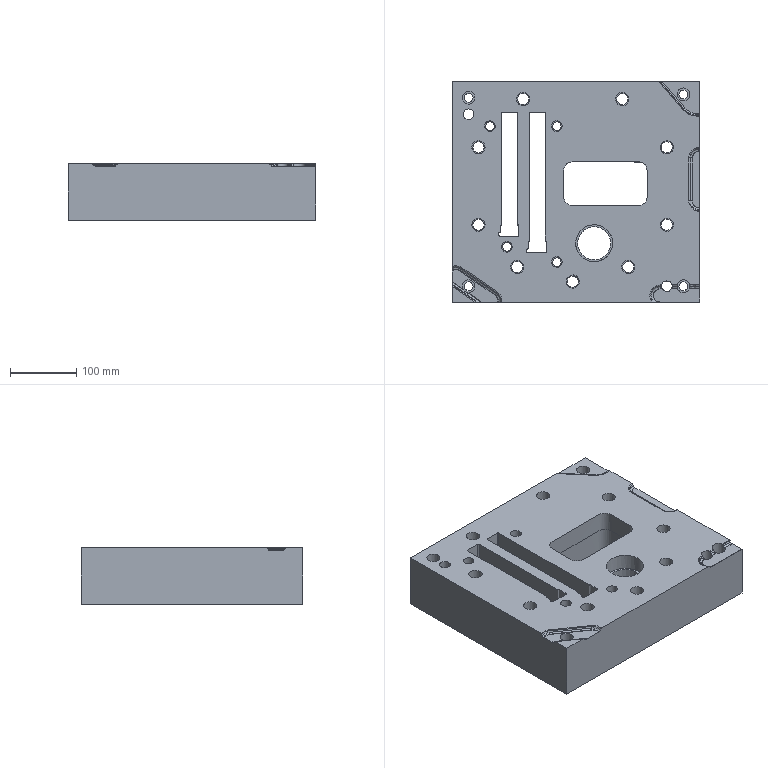Part | NX | features solid 2 | 1 solid | 145 faces | box 375.001 x 335.008 x 85 mm | volume 8450093 mm3 | spline 78 | cylinder 38 | plane 29 | commonest cylinder face diameters 17 x9 20 x9 16 x6 13 x4 13.5 x4 19.5 x4